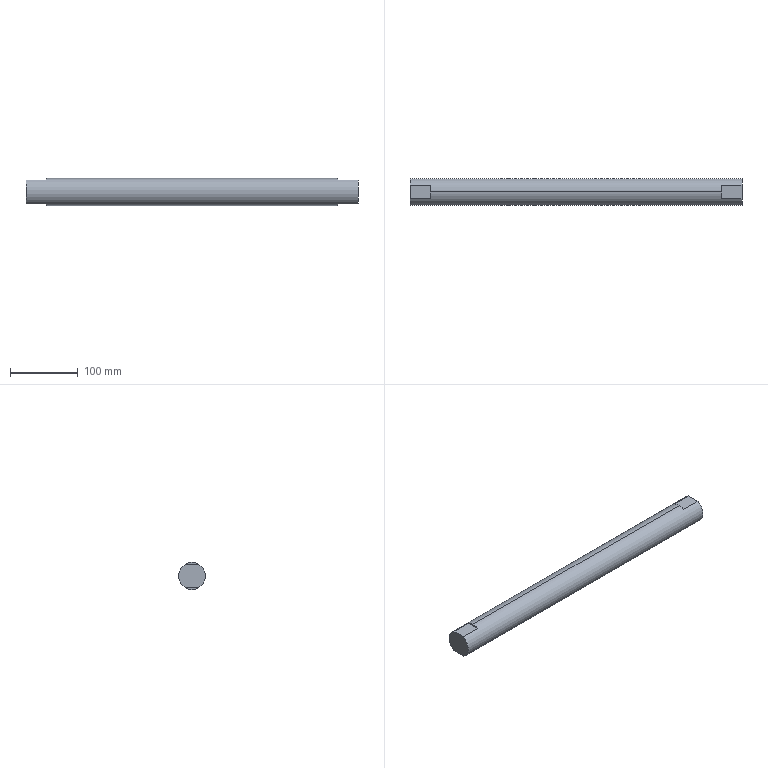Part | STEP file | Threading sliding shaft SGN-2-12 | 1 solid | 12 faces | box 490 x 40 x 40 mm | volume 611828 mm3 | plane 10 | cylinder 2 | commonest cylinder face diameters 40 x2
STEP:
#1=CARTESIAN_POINT('',(0.,0.,0.));
#2=DIRECTION('',(0.,0.,1.));
#3=DIRECTION('',(1.,0.,0.));
#4=AXIS2_PLACEMENT_3D('',#1,#2,#3);
#5=CARTESIAN_POINT('',(295.,9.682,-2.5));
#6=VERTEX_POINT('',#5);
#7=CARTESIAN_POINT('',(295.,0.,-5.));
#8=VERTEX_POINT('',#7);
#9=CARTESIAN_POINT('',(295.,0.,15.));
#10=DIRECTION('',(-1.,0.,0.));
#11=DIRECTION('',(0.,0.,-1.));
#12=AXIS2_PLACEMENT_3D('',#9,#10,#11);
#13=CIRCLE('',#12,20.);
#14=CARTESIAN_POINT('',(189.,0.,15.));
#15=DIRECTION('',(-1.,0.,0.));
#16=DIRECTION('',(0.,0.,1.));
#17=AXIS2_PLACEMENT_3D('',#14,#15,#16);
#18=CYLINDRICAL_SURFACE('',#17,20.);
#19=CARTESIAN_POINT('',(-3.142,-106.));
#20=DIRECTION('',(1.,0.));
#21=VECTOR('',#20,1.);
#22=LINE('',#19,#21);
#23=(GEOMETRIC_REPRESENTATION_CONTEXT(2)PARAMETRIC_REPRESENTATION_CONTEXT()REPRESENTATION_CONTEXT('',''));
#24=DEFINITIONAL_REPRESENTATION('',(#22),#23);
#25=PCURVE('',#18,#24);
#26=CARTESIAN_POINT('',(295.,0.,15.));
#27=DIRECTION('',(1.,0.,0.));
#28=DIRECTION('',(0.,0.,-1.));
#29=AXIS2_PLACEMENT_3D('',#26,#27,#28);
#30=PLANE('',#29);
#31=CARTESIAN_POINT('',(20.,0.));
#32=CARTESIAN_POINT('',(20.,-34.641));
#33=CARTESIAN_POINT('',(-10.,-17.321));
#34=CARTESIAN_POINT('',(-40.,0.));
#35=CARTESIAN_POINT('',(-10.,17.321));
#36=CARTESIAN_POINT('',(20.,34.641));
#37=CARTESIAN_POINT('',(20.,0.));
#38=(BOUNDED_CURVE()B_SPLINE_CURVE(2,(#31,#32,#33,#34,#35,#36,#37),.UNSPECIFIED.,.T.,.F.)B_SPLINE_CURVE_WITH_KNOTS((1,2,2,2,2,1),(-2.094,0.,2.094,4.189,6.283,8.378),.UNSPECIFIED.)CURVE()GEOMETRIC_REPRESENTATION_ITEM()RATIONAL_B_SPLINE_CURVE((1.,0.5,1.,0.5,1.,0.5,1.))REPRESENTATION_ITEM(''));
#39=(GEOMETRIC_REPRESENTATION_CONTEXT(2)PARAMETRIC_REPRESENTATION_CONTEXT()REPRESENTATION_CONTEXT('',''));
#40=DEFINITIONAL_REPRESENTATION('',(#38),#39);
#41=PCURVE('',#30,#40);
#42=SURFACE_CURVE('',#13,(#25,#41),.PCURVE_S1.);
#43=EDGE_CURVE('',#6,#8,#42,.T.);
#44=ORIENTED_EDGE('',*,*,#43,.T.);
#45=CARTESIAN_POINT('',(-135.,0.,-5.));
#46=VERTEX_POINT('',#45);
#47=CARTESIAN_POINT('',(189.,0.,-5.));
#48=DIRECTION('',(-1.,0.,0.));
#49=VECTOR('',#48,1.);
#50=LINE('',#47,#49);
#51=CARTESIAN_POINT('',(3.142,0.));
#52=DIRECTION('',(0.,1.));
#53=VECTOR('',#52,1.);
#54=LINE('',#51,#53);
#55=(GEOMETRIC_REPRESENTATION_CONTEXT(2)PARAMETRIC_REPRESENTATION_CONTEXT()REPRESENTATION_CONTEXT('',''));
#56=DEFINITIONAL_REPRESENTATION('',(#54),#55);
#57=PCURVE('',#18,#56);
#58=CARTESIAN_POINT('',(189.,0.,15.));
#59=DIRECTION('',(-1.,0.,0.));
#60=DIRECTION('',(0.,0.,1.));
#61=AXIS2_PLACEMENT_3D('',#58,#59,#60);
#62=CYLINDRICAL_SURFACE('',#61,20.);
#63=CARTESIAN_POINT('',(3.142,0.));
#64=DIRECTION('',(0.,1.));
#65=VECTOR('',#64,1.);
#66=LINE('',#63,#65);
#67=(GEOMETRIC_REPRESENTATION_CONTEXT(2)PARAMETRIC_REPRESENTATION_CONTEXT()REPRESENTATION_CONTEXT('',''));
#68=DEFINITIONAL_REPRESENTATION('',(#66),#67);
#69=PCURVE('',#62,#68);
#70=SURFACE_CURVE('',#50,(#57,#69),.PCURVE_S1.);
#71=EDGE_CURVE('',#8,#46,#70,.T.);
#72=ORIENTED_EDGE('',*,*,#71,.T.);
#73=CARTESIAN_POINT('',(-135.,9.682,-2.5));
#74=VERTEX_POINT('',#73);
#75=CARTESIAN_POINT('',(-135.,0.,15.));
#76=DIRECTION('',(1.,0.,0.));
#77=DIRECTION('',(0.,0.,1.));
#78=AXIS2_PLACEMENT_3D('',#75,#76,#77);
#79=CIRCLE('',#78,20.);
#80=CARTESIAN_POINT('',(6.283,324.));
#81=DIRECTION('',(-1.,0.));
#82=VECTOR('',#81,1.);
#83=LINE('',#80,#82);
#84=(GEOMETRIC_REPRESENTATION_CONTEXT(2)PARAMETRIC_REPRESENTATION_CONTEXT()REPRESENTATION_CONTEXT('',''));
#85=DEFINITIONAL_REPRESENTATION('',(#83),#84);
#86=PCURVE('',#18,#85);
#87=CARTESIAN_POINT('',(-135.,0.,15.));
#88=DIRECTION('',(-1.,0.,0.));
#89=DIRECTION('',(0.,0.,1.));
#90=AXIS2_PLACEMENT_3D('',#87,#88,#89);
#91=PLANE('',#90);
#92=CARTESIAN_POINT('',(20.,0.));
#93=CARTESIAN_POINT('',(20.,-34.641));
#94=CARTESIAN_POINT('',(-10.,-17.321));
#95=CARTESIAN_POINT('',(-40.,0.));
#96=CARTESIAN_POINT('',(-10.,17.321));
#97=CARTESIAN_POINT('',(20.,34.641));
#98=CARTESIAN_POINT('',(20.,0.));
#99=(BOUNDED_CURVE()B_SPLINE_CURVE(2,(#92,#93,#94,#95,#96,#97,#98),.UNSPECIFIED.,.T.,.F.)B_SPLINE_CURVE_WITH_KNOTS((1,2,2,2,2,1),(-2.094,0.,2.094,4.189,6.283,8.378),.UNSPECIFIED.)CURVE()GEOMETRIC_REPRESENTATION_ITEM()RATIONAL_B_SPLINE_CURVE((1.,0.5,1.,0.5,1.,0.5,1.))REPRESENTATION_ITEM(''));
#100=(GEOMETRIC_REPRESENTATION_CONTEXT(2)PARAMETRIC_REPRESENTATION_CONTEXT()REPRESENTATION_CONTEXT('',''));
#101=DEFINITIONAL_REPRESENTATION('',(#99),#100);
#102=PCURVE('',#91,#101);
#103=SURFACE_CURVE('',#79,(#86,#102),.PCURVE_S1.);
#104=EDGE_CURVE('',#46,#74,#103,.T.);
#105=ORIENTED_EDGE('',*,*,#104,.T.);
#106=CARTESIAN_POINT('',(-165.,9.682,-2.5));
#107=VERTEX_POINT('',#106);
#108=CARTESIAN_POINT('',(189.,9.682,-2.5));
#109=DIRECTION('',(-1.,0.,0.));
#110=VECTOR('',#109,1.);
#111=LINE('',#108,#110);
#112=CARTESIAN_POINT('',(2.636,0.));
#113=DIRECTION('',(0.,1.));
#114=VECTOR('',#113,1.);
#115=LINE('',#112,#114);
#116=(GEOMETRIC_REPRESENTATION_CONTEXT(2)PARAMETRIC_REPRESENTATION_CONTEXT()REPRESENTATION_CONTEXT('',''));
#117=DEFINITIONAL_REPRESENTATION('',(#115),#116);
#118=PCURVE('',#18,#117);
#119=CARTESIAN_POINT('',(-135.,-24.484,-2.5));
#120=DIRECTION('',(0.,0.,-1.));
#121=DIRECTION('',(-1.,0.,0.));
#122=AXIS2_PLACEMENT_3D('',#119,#120,#121);
#123=PLANE('',#122);
#124=CARTESIAN_POINT('',(-324.,34.167));
#125=DIRECTION('',(1.,0.));
#126=VECTOR('',#125,1.);
#127=LINE('',#124,#126);
#128=(GEOMETRIC_REPRESENTATION_CONTEXT(2)PARAMETRIC_REPRESENTATION_CONTEXT()REPRESENTATION_CONTEXT('',''));
#129=DEFINITIONAL_REPRESENTATION('',(#127),#128);
#130=PCURVE('',#123,#129);
#131=SURFACE_CURVE('',#111,(#118,#130),.PCURVE_S1.);
#132=EDGE_CURVE('',#74,#107,#131,.T.);
#133=ORIENTED_EDGE('',*,*,#132,.T.);
#134=CARTESIAN_POINT('',(-165.,9.682,32.5));
#135=VERTEX_POINT('',#134);
#136=CARTESIAN_POINT('',(-165.,0.,15.));
#137=DIRECTION('',(-1.,0.,0.));
#138=DIRECTION('',(0.,0.,1.));
#139=AXIS2_PLACEMENT_3D('',#136,#137,#138);
#140=CIRCLE('',#139,20.);
#141=CARTESIAN_POINT('',(0.,354.));
#142=DIRECTION('',(1.,0.));
#143=VECTOR('',#142,1.);
#144=LINE('',#141,#143);
#145=(GEOMETRIC_REPRESENTATION_CONTEXT(2)PARAMETRIC_REPRESENTATION_CONTEXT()REPRESENTATION_CONTEXT('',''));
#146=DEFINITIONAL_REPRESENTATION('',(#144),#145);
#147=PCURVE('',#18,#146);
#148=CARTESIAN_POINT('',(-165.,0.,15.));
#149=DIRECTION('',(-1.,0.,0.));
#150=DIRECTION('',(0.,0.,1.));
#151=AXIS2_PLACEMENT_3D('',#148,#149,#150);
#152=PLANE('',#151);
#153=CARTESIAN_POINT('',(0.,0.));
#154=DIRECTION('',(1.,0.));
#155=AXIS2_PLACEMENT_2D('',#153,#154);
#156=CIRCLE('',#155,20.);
#157=(GEOMETRIC_REPRESENTATION_CONTEXT(2)PARAMETRIC_REPRESENTATION_CONTEXT()REPRESENTATION_CONTEXT('',''));
#158=DEFINITIONAL_REPRESENTATION('',(#156),#157);
#159=PCURVE('',#152,#158);
#160=SURFACE_CURVE('',#140,(#147,#159),.PCURVE_S1.);
#161=EDGE_CURVE('',#135,#107,#160,.T.);
#162=ORIENTED_EDGE('',*,*,#161,.F.);
#163=CARTESIAN_POINT('',(-135.,9.682,32.5));
#164=VERTEX_POINT('',#163);
#165=CARTESIAN_POINT('',(189.,9.682,32.5));
#166=DIRECTION('',(1.,0.,0.));
#167=VECTOR('',#166,1.);
#168=LINE('',#165,#167);
#169=CARTESIAN_POINT('',(0.5054,0.));
#170=DIRECTION('',(0.,-1.));
#171=VECTOR('',#170,1.);
#172=LINE('',#169,#171);
#173=(GEOMETRIC_REPRESENTATION_CONTEXT(2)PARAMETRIC_REPRESENTATION_CONTEXT()REPRESENTATION_CONTEXT('',''));
#174=DEFINITIONAL_REPRESENTATION('',(#172),#173);
#175=PCURVE('',#18,#174);
#176=CARTESIAN_POINT('',(-135.,-24.484,32.5));
#177=DIRECTION('',(0.,0.,1.));
#178=DIRECTION('',(1.,0.,0.));
#179=AXIS2_PLACEMENT_3D('',#176,#177,#178);
#180=PLANE('',#179);
#181=CARTESIAN_POINT('',(324.,34.167));
#182=DIRECTION('',(1.,0.));
#183=VECTOR('',#182,1.);
#184=LINE('',#181,#183);
#185=(GEOMETRIC_REPRESENTATION_CONTEXT(2)PARAMETRIC_REPRESENTATION_CONTEXT()REPRESENTATION_CONTEXT('',''));
#186=DEFINITIONAL_REPRESENTATION('',(#184),#185);
#187=PCURVE('',#180,#186);
#188=SURFACE_CURVE('',#168,(#175,#187),.PCURVE_S1.);
#189=EDGE_CURVE('',#135,#164,#188,.T.);
#190=ORIENTED_EDGE('',*,*,#189,.T.);
#191=CARTESIAN_POINT('',(-135.,0.,35.));
#192=VERTEX_POINT('',#191);
#193=CARTESIAN_POINT('',(-135.,0.,15.));
#194=DIRECTION('',(1.,0.,0.));
#195=DIRECTION('',(0.,0.,1.));
#196=AXIS2_PLACEMENT_3D('',#193,#194,#195);
#197=CIRCLE('',#196,20.);
#198=CARTESIAN_POINT('',(6.283,324.));
#199=DIRECTION('',(-1.,0.));
#200=VECTOR('',#199,1.);
#201=LINE('',#198,#200);
#202=(GEOMETRIC_REPRESENTATION_CONTEXT(2)PARAMETRIC_REPRESENTATION_CONTEXT()REPRESENTATION_CONTEXT('',''));
#203=DEFINITIONAL_REPRESENTATION('',(#201),#202);
#204=PCURVE('',#18,#203);
#205=CARTESIAN_POINT('',(-135.,0.,15.));
#206=DIRECTION('',(-1.,0.,0.));
#207=DIRECTION('',(0.,0.,1.));
#208=AXIS2_PLACEMENT_3D('',#205,#206,#207);
#209=PLANE('',#208);
#210=CARTESIAN_POINT('',(20.,0.));
#211=CARTESIAN_POINT('',(20.,-34.641));
#212=CARTESIAN_POINT('',(-10.,-17.321));
#213=CARTESIAN_POINT('',(-40.,0.));
#214=CARTESIAN_POINT('',(-10.,17.321));
#215=CARTESIAN_POINT('',(20.,34.641));
#216=CARTESIAN_POINT('',(20.,0.));
#217=(BOUNDED_CURVE()B_SPLINE_CURVE(2,(#210,#211,#212,#213,#214,#215,#216),.UNSPECIFIED.,.T.,.F.)B_SPLINE_CURVE_WITH_KNOTS((1,2,2,2,2,1),(-2.094,0.,2.094,4.189,6.283,8.378),.UNSPECIFIED.)CURVE()GEOMETRIC_REPRESENTATION_ITEM()RATIONAL_B_SPLINE_CURVE((1.,0.5,1.,0.5,1.,0.5,1.))REPRESENTATION_ITEM(''));
#218=(GEOMETRIC_REPRESENTATION_CONTEXT(2)PARAMETRIC_REPRESENTATION_CONTEXT()REPRESENTATION_CONTEXT('',''));
#219=DEFINITIONAL_REPRESENTATION('',(#217),#218);
#220=PCURVE('',#209,#219);
#221=SURFACE_CURVE('',#197,(#204,#220),.PCURVE_S1.);
#222=EDGE_CURVE('',#164,#192,#221,.T.);
#223=ORIENTED_EDGE('',*,*,#222,.T.);
#224=CARTESIAN_POINT('',(295.,0.,35.));
#225=VERTEX_POINT('',#224);
#226=CARTESIAN_POINT('',(189.,0.,35.));
#227=DIRECTION('',(-1.,0.,0.));
#228=VECTOR('',#227,1.);
#229=LINE('',#226,#228);
#230=CARTESIAN_POINT('',(0.,0.));
#231=DIRECTION('',(0.,1.));
#232=VECTOR('',#231,1.);
#233=LINE('',#230,#232);
#234=(GEOMETRIC_REPRESENTATION_CONTEXT(2)PARAMETRIC_REPRESENTATION_CONTEXT()REPRESENTATION_CONTEXT('',''));
#235=DEFINITIONAL_REPRESENTATION('',(#233),#234);
#236=PCURVE('',#18,#235);
#237=CARTESIAN_POINT('',(6.283,0.));
#238=DIRECTION('',(0.,1.));
#239=VECTOR('',#238,1.);
#240=LINE('',#237,#239);
#241=(GEOMETRIC_REPRESENTATION_CONTEXT(2)PARAMETRIC_REPRESENTATION_CONTEXT()REPRESENTATION_CONTEXT('',''));
#242=DEFINITIONAL_REPRESENTATION('',(#240),#241);
#243=PCURVE('',#62,#242);
#244=SURFACE_CURVE('',#229,(#236,#243),.PCURVE_S1.);
#245=EDGE_CURVE('',#225,#192,#244,.T.);
#246=ORIENTED_EDGE('',*,*,#245,.F.);
#247=CARTESIAN_POINT('',(295.,9.682,32.5));
#248=VERTEX_POINT('',#247);
#249=CARTESIAN_POINT('',(295.,0.,15.));
#250=DIRECTION('',(-1.,0.,0.));
#251=DIRECTION('',(0.,0.,-1.));
#252=AXIS2_PLACEMENT_3D('',#249,#250,#251);
#253=CIRCLE('',#252,20.);
#254=CARTESIAN_POINT('',(-3.142,-106.));
#255=DIRECTION('',(1.,0.));
#256=VECTOR('',#255,1.);
#257=LINE('',#254,#256);
#258=(GEOMETRIC_REPRESENTATION_CONTEXT(2)PARAMETRIC_REPRESENTATION_CONTEXT()REPRESENTATION_CONTEXT('',''));
#259=DEFINITIONAL_REPRESENTATION('',(#257),#258);
#260=PCURVE('',#18,#259);
#261=CARTESIAN_POINT('',(295.,0.,15.));
#262=DIRECTION('',(1.,0.,0.));
#263=DIRECTION('',(0.,0.,-1.));
#264=AXIS2_PLACEMENT_3D('',#261,#262,#263);
#265=PLANE('',#264);
#266=CARTESIAN_POINT('',(20.,0.));
#267=CARTESIAN_POINT('',(20.,-34.641));
#268=CARTESIAN_POINT('',(-10.,-17.321));
#269=CARTESIAN_POINT('',(-40.,0.));
#270=CARTESIAN_POINT('',(-10.,17.321));
#271=CARTESIAN_POINT('',(20.,34.641));
#272=CARTESIAN_POINT('',(20.,0.));
#273=(BOUNDED_CURVE()B_SPLINE_CURVE(2,(#266,#267,#268,#269,#270,#271,#272),.UNSPECIFIED.,.T.,.F.)B_SPLINE_CURVE_WITH_KNOTS((1,2,2,2,2,1),(-2.094,0.,2.094,4.189,6.283,8.378),.UNSPECIFIED.)CURVE()GEOMETRIC_REPRESENTATION_ITEM()RATIONAL_B_SPLINE_CURVE((1.,0.5,1.,0.5,1.,0.5,1.))REPRESENTATION_ITEM(''));
#274=(GEOMETRIC_REPRESENTATION_CONTEXT(2)PARAMETRIC_REPRESENTATION_CONTEXT()REPRESENTATION_CONTEXT('',''));
#275=DEFINITIONAL_REPRESENTATION('',(#273),#274);
#276=PCURVE('',#265,#275);
#277=SURFACE_CURVE('',#253,(#260,#276),.PCURVE_S1.);
#278=EDGE_CURVE('',#225,#248,#277,.T.);
#279=ORIENTED_EDGE('',*,*,#278,.T.);
#280=CARTESIAN_POINT('',(325.,9.682,32.5));
#281=VERTEX_POINT('',#280);
#282=CARTESIAN_POINT('',(189.,9.682,32.5));
#283=DIRECTION('',(1.,0.,0.));
#284=VECTOR('',#283,1.);
#285=LINE('',#282,#284);
#286=CARTESIAN_POINT('',(0.5054,0.));
#287=DIRECTION('',(0.,-1.));
#288=VECTOR('',#287,1.);
#289=LINE('',#286,#288);
#290=(GEOMETRIC_REPRESENTATION_CONTEXT(2)PARAMETRIC_REPRESENTATION_CONTEXT()REPRESENTATION_CONTEXT('',''));
#291=DEFINITIONAL_REPRESENTATION('',(#289),#290);
#292=PCURVE('',#18,#291);
#293=CARTESIAN_POINT('',(295.,-22.774,32.5));
#294=DIRECTION('',(0.,0.,1.));
#295=DIRECTION('',(1.,0.,0.));
#296=AXIS2_PLACEMENT_3D('',#293,#294,#295);
#297=PLANE('',#296);
#298=CARTESIAN_POINT('',(-106.,32.457));
#299=DIRECTION('',(1.,0.));
#300=VECTOR('',#299,1.);
#301=LINE('',#298,#300);
#302=(GEOMETRIC_REPRESENTATION_CONTEXT(2)PARAMETRIC_REPRESENTATION_CONTEXT()REPRESENTATION_CONTEXT('',''));
#303=DEFINITIONAL_REPRESENTATION('',(#301),#302);
#304=PCURVE('',#297,#303);
#305=SURFACE_CURVE('',#285,(#292,#304),.PCURVE_S1.);
#306=EDGE_CURVE('',#248,#281,#305,.T.);
#307=ORIENTED_EDGE('',*,*,#306,.T.);
#308=CARTESIAN_POINT('',(325.,9.682,-2.5));
#309=VERTEX_POINT('',#308);
#310=CARTESIAN_POINT('',(325.,0.,15.));
#311=DIRECTION('',(1.,0.,0.));
#312=DIRECTION('',(0.,0.,-1.));
#313=AXIS2_PLACEMENT_3D('',#310,#311,#312);
#314=CIRCLE('',#313,20.);
#315=CARTESIAN_POINT('',(3.142,-136.));
#316=DIRECTION('',(-1.,0.));
#317=VECTOR('',#316,1.);
#318=LINE('',#315,#317);
#319=(GEOMETRIC_REPRESENTATION_CONTEXT(2)PARAMETRIC_REPRESENTATION_CONTEXT()REPRESENTATION_CONTEXT('',''));
#320=DEFINITIONAL_REPRESENTATION('',(#318),#319);
#321=PCURVE('',#18,#320);
#322=CARTESIAN_POINT('',(325.,0.,15.));
#323=DIRECTION('',(1.,0.,0.));
#324=DIRECTION('',(0.,0.,-1.));
#325=AXIS2_PLACEMENT_3D('',#322,#323,#324);
#326=PLANE('',#325);
#327=CARTESIAN_POINT('',(0.,0.));
#328=DIRECTION('',(1.,0.));
#329=AXIS2_PLACEMENT_2D('',#327,#328);
#330=CIRCLE('',#329,20.);
#331=(GEOMETRIC_REPRESENTATION_CONTEXT(2)PARAMETRIC_REPRESENTATION_CONTEXT()REPRESENTATION_CONTEXT('',''));
#332=DEFINITIONAL_REPRESENTATION('',(#330),#331);
#333=PCURVE('',#326,#332);
#334=SURFACE_CURVE('',#314,(#321,#333),.PCURVE_S1.);
#335=EDGE_CURVE('',#309,#281,#334,.T.);
#336=ORIENTED_EDGE('',*,*,#335,.F.);
#337=CARTESIAN_POINT('',(189.,9.682,-2.5));
#338=DIRECTION('',(-1.,0.,0.));
#339=VECTOR('',#338,1.);
#340=LINE('',#337,#339);
#341=CARTESIAN_POINT('',(2.636,0.));
#342=DIRECTION('',(0.,1.));
#343=VECTOR('',#342,1.);
#344=LINE('',#341,#343);
#345=(GEOMETRIC_REPRESENTATION_CONTEXT(2)PARAMETRIC_REPRESENTATION_CONTEXT()REPRESENTATION_CONTEXT('',''));
#346=DEFINITIONAL_REPRESENTATION('',(#344),#345);
#347=PCURVE('',#18,#346);
#348=CARTESIAN_POINT('',(295.,-22.774,-2.5));
#349=DIRECTION('',(0.,0.,-1.));
#350=DIRECTION('',(-1.,0.,0.));
#351=AXIS2_PLACEMENT_3D('',#348,#349,#350);
#352=PLANE('',#351);
#353=CARTESIAN_POINT('',(106.,32.457));
#354=DIRECTION('',(1.,0.));
#355=VECTOR('',#354,1.);
#356=LINE('',#353,#355);
#357=(GEOMETRIC_REPRESENTATION_CONTEXT(2)PARAMETRIC_REPRESENTATION_CONTEXT()REPRESENTATION_CONTEXT('',''));
#358=DEFINITIONAL_REPRESENTATION('',(#356),#357);
#359=PCURVE('',#352,#358);
#360=SURFACE_CURVE('',#340,(#347,#359),.PCURVE_S1.);
#361=EDGE_CURVE('',#309,#6,#360,.T.);
#362=ORIENTED_EDGE('',*,*,#361,.T.);
#363=EDGE_LOOP('',(#44,#72,#105,#133,#162,#190,#223,#246,#279,#307,#336,#362));
#364=FACE_BOUND('',#363,.T.);
#365=ADVANCED_FACE('',(#364),#18,.T.);
#366=ORIENTED_EDGE('',*,*,#71,.F.);
#367=CARTESIAN_POINT('',(295.,-9.682,-2.5));
#368=VERTEX_POINT('',#367);
#369=CARTESIAN_POINT('',(295.,0.,15.));
#370=DIRECTION('',(-1.,0.,0.));
#371=DIRECTION('',(0.,0.,-1.));
#372=AXIS2_PLACEMENT_3D('',#369,#370,#371);
#373=CIRCLE('',#372,20.);
#374=CARTESIAN_POINT('',(3.142,-106.));
#375=DIRECTION('',(1.,0.));
#376=VECTOR('',#375,1.);
#377=LINE('',#374,#376);
#378=(GEOMETRIC_REPRESENTATION_CONTEXT(2)PARAMETRIC_REPRESENTATION_CONTEXT()REPRESENTATION_CONTEXT('',''));
#379=DEFINITIONAL_REPRESENTATION('',(#377),#378);
#380=PCURVE('',#62,#379);
#381=CARTESIAN_POINT('',(20.,0.));
#382=CARTESIAN_POINT('',(20.,-34.641));
#383=CARTESIAN_POINT('',(-10.,-17.321));
#384=CARTESIAN_POINT('',(-40.,0.));
#385=CARTESIAN_POINT('',(-10.,17.321));
#386=CARTESIAN_POINT('',(20.,34.641));
#387=CARTESIAN_POINT('',(20.,0.));
#388=(BOUNDED_CURVE()B_SPLINE_CURVE(2,(#381,#382,#383,#384,#385,#386,#387),.UNSPECIFIED.,.T.,.F.)B_SPLINE_CURVE_WITH_KNOTS((1,2,2,2,2,1),(-2.094,0.,2.094,4.189,6.283,8.378),.UNSPECIFIED.)CURVE()GEOMETRIC_REPRESENTATION_ITEM()RATIONAL_B_SPLINE_CURVE((1.,0.5,1.,0.5,1.,0.5,1.))REPRESENTATION_ITEM(''));
#389=(GEOMETRIC_REPRESENTATION_CONTEXT(2)PARAMETRIC_REPRESENTATION_CONTEXT()REPRESENTATION_CONTEXT('',''));
#390=DEFINITIONAL_REPRESENTATION('',(#388),#389);
#391=PCURVE('',#30,#390);
#392=SURFACE_CURVE('',#373,(#380,#391),.PCURVE_S1.);
#393=EDGE_CURVE('',#8,#368,#392,.T.);
#394=ORIENTED_EDGE('',*,*,#393,.T.);
#395=CARTESIAN_POINT('',(325.,-9.682,-2.5));
#396=VERTEX_POINT('',#395);
#397=CARTESIAN_POINT('',(189.,-9.682,-2.5));
#398=DIRECTION('',(1.,0.,0.));
#399=VECTOR('',#398,1.);
#400=LINE('',#397,#399);
#401=CARTESIAN_POINT('',(3.647,0.));
#402=DIRECTION('',(0.,-1.));
#403=VECTOR('',#402,1.);
#404=LINE('',#401,#403);
#405=(GEOMETRIC_REPRESENTATION_CONTEXT(2)PARAMETRIC_REPRESENTATION_CONTEXT()REPRESENTATION_CONTEXT('',''));
#406=DEFINITIONAL_REPRESENTATION('',(#404),#405);
#407=PCURVE('',#62,#406);
#408=CARTESIAN_POINT('',(106.,13.092));
#409=DIRECTION('',(-1.,0.));
#410=VECTOR('',#409,1.);
#411=LINE('',#408,#410);
#412=(GEOMETRIC_REPRESENTATION_CONTEXT(2)PARAMETRIC_REPRESENTATION_CONTEXT()REPRESENTATION_CONTEXT('',''));
#413=DEFINITIONAL_REPRESENTATION('',(#411),#412);
#414=PCURVE('',#352,#413);
#415=SURFACE_CURVE('',#400,(#407,#414),.PCURVE_S1.);
#416=EDGE_CURVE('',#368,#396,#415,.T.);
#417=ORIENTED_EDGE('',*,*,#416,.T.);
#418=CARTESIAN_POINT('',(325.,-9.682,32.5));
#419=VERTEX_POINT('',#418);
#420=CARTESIAN_POINT('',(325.,0.,15.));
#421=DIRECTION('',(1.,0.,0.));
#422=DIRECTION('',(0.,0.,-1.));
#423=AXIS2_PLACEMENT_3D('',#420,#421,#422);
#424=CIRCLE('',#423,20.);
#425=CARTESIAN_POINT('',(9.425,-136.));
#426=DIRECTION('',(-1.,0.));
#427=VECTOR('',#426,1.);
#428=LINE('',#425,#427);
#429=(GEOMETRIC_REPRESENTATION_CONTEXT(2)PARAMETRIC_REPRESENTATION_CONTEXT()REPRESENTATION_CONTEXT('',''));
#430=DEFINITIONAL_REPRESENTATION('',(#428),#429);
#431=PCURVE('',#62,#430);
#432=CARTESIAN_POINT('',(0.,0.));
#433=DIRECTION('',(1.,0.));
#434=AXIS2_PLACEMENT_2D('',#432,#433);
#435=CIRCLE('',#434,20.);
#436=(GEOMETRIC_REPRESENTATION_CONTEXT(2)PARAMETRIC_REPRESENTATION_CONTEXT()REPRESENTATION_CONTEXT('',''));
#437=DEFINITIONAL_REPRESENTATION('',(#435),#436);
#438=PCURVE('',#326,#437);
#439=SURFACE_CURVE('',#424,(#431,#438),.PCURVE_S1.);
#440=EDGE_CURVE('',#419,#396,#439,.T.);
#441=ORIENTED_EDGE('',*,*,#440,.F.);
#442=CARTESIAN_POINT('',(295.,-9.682,32.5));
#443=VERTEX_POINT('',#442);
#444=CARTESIAN_POINT('',(189.,-9.682,32.5));
#445=DIRECTION('',(-1.,0.,0.));
#446=VECTOR('',#445,1.);
#447=LINE('',#444,#446);
#448=CARTESIAN_POINT('',(5.778,0.));
#449=DIRECTION('',(0.,1.));
#450=VECTOR('',#449,1.);
#451=LINE('',#448,#450);
#452=(GEOMETRIC_REPRESENTATION_CONTEXT(2)PARAMETRIC_REPRESENTATION_CONTEXT()REPRESENTATION_CONTEXT('',''));
#453=DEFINITIONAL_REPRESENTATION('',(#451),#452);
#454=PCURVE('',#62,#453);
#455=CARTESIAN_POINT('',(-106.,13.092));
#456=DIRECTION('',(-1.,0.));
#457=VECTOR('',#456,1.);
#458=LINE('',#455,#457);
#459=(GEOMETRIC_REPRESENTATION_CONTEXT(2)PARAMETRIC_REPRESENTATION_CONTEXT()REPRESENTATION_CONTEXT('',''));
#460=DEFINITIONAL_REPRESENTATION('',(#458),#459);
#461=PCURVE('',#297,#460);
#462=SURFACE_CURVE('',#447,(#454,#461),.PCURVE_S1.);
#463=EDGE_CURVE('',#419,#443,#462,.T.);
#464=ORIENTED_EDGE('',*,*,#463,.T.);
#465=CARTESIAN_POINT('',(295.,0.,15.));
#466=DIRECTION('',(-1.,0.,0.));
#467=DIRECTION('',(0.,0.,-1.));
#468=AXIS2_PLACEMENT_3D('',#465,#466,#467);
#469=CIRCLE('',#468,20.);
#470=CARTESIAN_POINT('',(3.142,-106.));
#471=DIRECTION('',(1.,0.));
#472=VECTOR('',#471,1.);
#473=LINE('',#470,#472);
#474=(GEOMETRIC_REPRESENTATION_CONTEXT(2)PARAMETRIC_REPRESENTATION_CONTEXT()REPRESENTATION_CONTEXT('',''));
#475=DEFINITIONAL_REPRESENTATION('',(#473),#474);
#476=PCURVE('',#62,#475);
#477=CARTESIAN_POINT('',(20.,0.));
#478=CARTESIAN_POINT('',(20.,-34.641));
#479=CARTESIAN_POINT('',(-10.,-17.321));
#480=CARTESIAN_POINT('',(-40.,0.));
#481=CARTESIAN_POINT('',(-10.,17.321));
#482=CARTESIAN_POINT('',(20.,34.641));
#483=CARTESIAN_POINT('',(20.,0.));
#484=(BOUNDED_CURVE()B_SPLINE_CURVE(2,(#477,#478,#479,#480,#481,#482,#483),.UNSPECIFIED.,.T.,.F.)B_SPLINE_CURVE_WITH_KNOTS((1,2,2,2,2,1),(-2.094,0.,2.094,4.189,6.283,8.378),.UNSPECIFIED.)CURVE()GEOMETRIC_REPRESENTATION_ITEM()RATIONAL_B_SPLINE_CURVE((1.,0.5,1.,0.5,1.,0.5,1.))REPRESENTATION_ITEM(''));
#485=(GEOMETRIC_REPRESENTATION_CONTEXT(2)PARAMETRIC_REPRESENTATION_CONTEXT()REPRESENTATION_CONTEXT('',''));
#486=DEFINITIONAL_REPRESENTATION('',(#484),#485);
#487=PCURVE('',#265,#486);
#488=SURFACE_CURVE('',#469,(#476,#487),.PCURVE_S1.);
#489=EDGE_CURVE('',#443,#225,#488,.T.);
#490=ORIENTED_EDGE('',*,*,#489,.T.);
#491=ORIENTED_EDGE('',*,*,#245,.T.);
#492=CARTESIAN_POINT('',(-135.,-9.682,32.5));
#493=VERTEX_POINT('',#492);
#494=CARTESIAN_POINT('',(-135.,0.,15.));
#495=DIRECTION('',(1.,0.,0.));
#496=DIRECTION('',(0.,0.,1.));
#497=AXIS2_PLACEMENT_3D('',#494,#495,#496);
#498=CIRCLE('',#497,20.);
#499=CARTESIAN_POINT('',(6.283,324.));
#500=DIRECTION('',(-1.,0.));
#501=VECTOR('',#500,1.);
#502=LINE('',#499,#501);
#503=(GEOMETRIC_REPRESENTATION_CONTEXT(2)PARAMETRIC_REPRESENTATION_CONTEXT()REPRESENTATION_CONTEXT('',''));
#504=DEFINITIONAL_REPRESENTATION('',(#502),#503);
#505=PCURVE('',#62,#504);
#506=CARTESIAN_POINT('',(20.,0.));
#507=CARTESIAN_POINT('',(20.,-34.641));
#508=CARTESIAN_POINT('',(-10.,-17.321));
#509=CARTESIAN_POINT('',(-40.,0.));
#510=CARTESIAN_POINT('',(-10.,17.321));
#511=CARTESIAN_POINT('',(20.,34.641));
#512=CARTESIAN_POINT('',(20.,0.));
#513=(BOUNDED_CURVE()B_SPLINE_CURVE(2,(#506,#507,#508,#509,#510,#511,#512),.UNSPECIFIED.,.T.,.F.)B_SPLINE_CURVE_WITH_KNOTS((1,2,2,2,2,1),(-2.094,0.,2.094,4.189,6.283,8.378),.UNSPECIFIED.)CURVE()GEOMETRIC_REPRESENTATION_ITEM()RATIONAL_B_SPLINE_CURVE((1.,0.5,1.,0.5,1.,0.5,1.))REPRESENTATION_ITEM(''));
#514=(GEOMETRIC_REPRESENTATION_CONTEXT(2)PARAMETRIC_REPRESENTATION_CONTEXT()REPRESENTATION_CONTEXT('',''));
#515=DEFINITIONAL_REPRESENTATION('',(#513),#514);
#516=PCURVE('',#209,#515);
#517=SURFACE_CURVE('',#498,(#505,#516),.PCURVE_S1.);
#518=EDGE_CURVE('',#192,#493,#517,.T.);
#519=ORIENTED_EDGE('',*,*,#518,.T.);
#520=CARTESIAN_POINT('',(-165.,-9.682,32.5));
#521=VERTEX_POINT('',#520);
#522=CARTESIAN_POINT('',(189.,-9.682,32.5));
#523=DIRECTION('',(-1.,0.,0.));
#524=VECTOR('',#523,1.);
#525=LINE('',#522,#524);
#526=CARTESIAN_POINT('',(5.778,0.));
#527=DIRECTION('',(0.,1.));
#528=VECTOR('',#527,1.);
#529=LINE('',#526,#528);
#530=(GEOMETRIC_REPRESENTATION_CONTEXT(2)PARAMETRIC_REPRESENTATION_CONTEXT()REPRESENTATION_CONTEXT('',''));
#531=DEFINITIONAL_REPRESENTATION('',(#529),#530);
#532=PCURVE('',#62,#531);
#533=CARTESIAN_POINT('',(324.,14.802));
#534=DIRECTION('',(-1.,0.));
#535=VECTOR('',#534,1.);
#536=LINE('',#533,#535);
#537=(GEOMETRIC_REPRESENTATION_CONTEXT(2)PARAMETRIC_REPRESENTATION_CONTEXT()REPRESENTATION_CONTEXT('',''));
#538=DEFINITIONAL_REPRESENTATION('',(#536),#537);
#539=PCURVE('',#180,#538);
#540=SURFACE_CURVE('',#525,(#532,#539),.PCURVE_S1.);
#541=EDGE_CURVE('',#493,#521,#540,.T.);
#542=ORIENTED_EDGE('',*,*,#541,.T.);
#543=CARTESIAN_POINT('',(-165.,-9.682,-2.5));
#544=VERTEX_POINT('',#543);
#545=CARTESIAN_POINT('',(-165.,0.,15.));
#546=DIRECTION('',(-1.,0.,0.));
#547=DIRECTION('',(0.,0.,1.));
#548=AXIS2_PLACEMENT_3D('',#545,#546,#547);
#549=CIRCLE('',#548,20.);
#550=CARTESIAN_POINT('',(0.,354.));
#551=DIRECTION('',(1.,0.));
#552=VECTOR('',#551,1.);
#553=LINE('',#550,#552);
#554=(GEOMETRIC_REPRESENTATION_CONTEXT(2)PARAMETRIC_REPRESENTATION_CONTEXT()REPRESENTATION_CONTEXT('',''));
#555=DEFINITIONAL_REPRESENTATION('',(#553),#554);
#556=PCURVE('',#62,#555);
#557=CARTESIAN_POINT('',(0.,0.));
#558=DIRECTION('',(1.,0.));
#559=AXIS2_PLACEMENT_2D('',#557,#558);
#560=CIRCLE('',#559,20.);
#561=(GEOMETRIC_REPRESENTATION_CONTEXT(2)PARAMETRIC_REPRESENTATION_CONTEXT()REPRESENTATION_CONTEXT('',''));
#562=DEFINITIONAL_REPRESENTATION('',(#560),#561);
#563=PCURVE('',#152,#562);
#564=SURFACE_CURVE('',#549,(#556,#563),.PCURVE_S1.);
#565=EDGE_CURVE('',#544,#521,#564,.T.);
#566=ORIENTED_EDGE('',*,*,#565,.F.);
#567=CARTESIAN_POINT('',(-135.,-9.682,-2.5));
#568=VERTEX_POINT('',#567);
#569=CARTESIAN_POINT('',(189.,-9.682,-2.5));
#570=DIRECTION('',(1.,0.,0.));
#571=VECTOR('',#570,1.);
#572=LINE('',#569,#571);
#573=CARTESIAN_POINT('',(3.647,0.));
#574=DIRECTION('',(0.,-1.));
#575=VECTOR('',#574,1.);
#576=LINE('',#573,#575);
#577=(GEOMETRIC_REPRESENTATION_CONTEXT(2)PARAMETRIC_REPRESENTATION_CONTEXT()REPRESENTATION_CONTEXT('',''));
#578=DEFINITIONAL_REPRESENTATION('',(#576),#577);
#579=PCURVE('',#62,#578);
#580=CARTESIAN_POINT('',(-324.,14.802));
#581=DIRECTION('',(-1.,0.));
#582=VECTOR('',#581,1.);
#583=LINE('',#580,#582);
#584=(GEOMETRIC_REPRESENTATION_CONTEXT(2)PARAMETRIC_REPRESENTATION_CONTEXT()REPRESENTATION_CONTEXT('',''));
#585=DEFINITIONAL_REPRESENTATION('',(#583),#584);
#586=PCURVE('',#123,#585);
#587=SURFACE_CURVE('',#572,(#579,#586),.PCURVE_S1.);
#588=EDGE_CURVE('',#544,#568,#587,.T.);
#589=ORIENTED_EDGE('',*,*,#588,.T.);
#590=CARTESIAN_POINT('',(-135.,0.,15.));
#591=DIRECTION('',(1.,0.,0.));
#592=DIRECTION('',(0.,0.,1.));
#593=AXIS2_PLACEMENT_3D('',#590,#591,#592);
#594=CIRCLE('',#593,20.);
#595=CARTESIAN_POINT('',(6.283,324.));
#596=DIRECTION('',(-1.,0.));
#597=VECTOR('',#596,1.);
#598=LINE('',#595,#597);
#599=(GEOMETRIC_REPRESENTATION_CONTEXT(2)PARAMETRIC_REPRESENTATION_CONTEXT()REPRESENTATION_CONTEXT('',''));
#600=DEFINITIONAL_REPRESENTATION('',(#598),#599);
#601=PCURVE('',#62,#600);
#602=CARTESIAN_POINT('',(20.,0.));
#603=CARTESIAN_POINT('',(20.,-34.641));
#604=CARTESIAN_POINT('',(-10.,-17.321));
#605=CARTESIAN_POINT('',(-40.,0.));
#606=CARTESIAN_POINT('',(-10.,17.321));
#607=CARTESIAN_POINT('',(20.,34.641));
#608=CARTESIAN_POINT('',(20.,0.));
#609=(BOUNDED_CURVE()B_SPLINE_CURVE(2,(#602,#603,#604,#605,#606,#607,#608),.UNSPECIFIED.,.T.,.F.)B_SPLINE_CURVE_WITH_KNOTS((1,2,2,2,2,1),(-2.094,0.,2.094,4.189,6.283,8.378),.UNSPECIFIED.)CURVE()GEOMETRIC_REPRESENTATION_ITEM()RATIONAL_B_SPLINE_CURVE((1.,0.5,1.,0.5,1.,0.5,1.))REPRESENTATION_ITEM(''));
#610=(GEOMETRIC_REPRESENTATION_CONTEXT(2)PARAMETRIC_REPRESENTATION_CONTEXT()REPRESENTATION_CONTEXT('',''));
#611=DEFINITIONAL_REPRESENTATION('',(#609),#610);
#612=PCURVE('',#91,#611);
#613=SURFACE_CURVE('',#594,(#601,#612),.PCURVE_S1.);
#614=EDGE_CURVE('',#568,#46,#613,.T.);
#615=ORIENTED_EDGE('',*,*,#614,.T.);
#616=EDGE_LOOP('',(#366,#394,#417,#441,#464,#490,#491,#519,#542,#566,#589,#615));
#617=FACE_BOUND('',#616,.T.);
#618=ADVANCED_FACE('',(#617),#62,.T.);
#619=ORIENTED_EDGE('',*,*,#565,.T.);
#620=CARTESIAN_POINT('',(-165.,0.,32.5));
#621=DIRECTION('',(0.,1.,0.));
#622=VECTOR('',#621,1.);
#623=LINE('',#620,#622);
#624=CARTESIAN_POINT('',(17.5,0.));
#625=DIRECTION('',(0.,1.));
#626=VECTOR('',#625,1.);
#627=LINE('',#624,#626);
#628=(GEOMETRIC_REPRESENTATION_CONTEXT(2)PARAMETRIC_REPRESENTATION_CONTEXT()REPRESENTATION_CONTEXT('',''));
#629=DEFINITIONAL_REPRESENTATION('',(#627),#628);
#630=PCURVE('',#152,#629);
#631=CARTESIAN_POINT('',(-30.,24.484));
#632=DIRECTION('',(0.,1.));
#633=VECTOR('',#632,1.);
#634=LINE('',#631,#633);
#635=(GEOMETRIC_REPRESENTATION_CONTEXT(2)PARAMETRIC_REPRESENTATION_CONTEXT()REPRESENTATION_CONTEXT('',''));
#636=DEFINITIONAL_REPRESENTATION('',(#634),#635);
#637=PCURVE('',#180,#636);
#638=SURFACE_CURVE('',#623,(#630,#637),.PCURVE_S1.);
#639=EDGE_CURVE('',#521,#135,#638,.T.);
#640=ORIENTED_EDGE('',*,*,#639,.T.);
#641=ORIENTED_EDGE('',*,*,#161,.T.);
#642=CARTESIAN_POINT('',(-165.,0.,-2.5));
#643=DIRECTION('',(0.,-1.,0.));
#644=VECTOR('',#643,1.);
#645=LINE('',#642,#644);
#646=CARTESIAN_POINT('',(-17.5,0.));
#647=DIRECTION('',(0.,-1.));
#648=VECTOR('',#647,1.);
#649=LINE('',#646,#648);
#650=(GEOMETRIC_REPRESENTATION_CONTEXT(2)PARAMETRIC_REPRESENTATION_CONTEXT()REPRESENTATION_CONTEXT('',''));
#651=DEFINITIONAL_REPRESENTATION('',(#649),#650);
#652=PCURVE('',#152,#651);
#653=CARTESIAN_POINT('',(30.,24.484));
#654=DIRECTION('',(0.,-1.));
#655=VECTOR('',#654,1.);
#656=LINE('',#653,#655);
#657=(GEOMETRIC_REPRESENTATION_CONTEXT(2)PARAMETRIC_REPRESENTATION_CONTEXT()REPRESENTATION_CONTEXT('',''));
#658=DEFINITIONAL_REPRESENTATION('',(#656),#657);
#659=PCURVE('',#123,#658);
#660=SURFACE_CURVE('',#645,(#652,#659),.PCURVE_S1.);
#661=EDGE_CURVE('',#107,#544,#660,.T.);
#662=ORIENTED_EDGE('',*,*,#661,.T.);
#663=EDGE_LOOP('',(#619,#640,#641,#662));
#664=FACE_BOUND('',#663,.T.);
#665=ADVANCED_FACE('',(#664),#152,.T.);
#666=ORIENTED_EDGE('',*,*,#440,.T.);
#667=CARTESIAN_POINT('',(325.,0.,-2.5));
#668=DIRECTION('',(0.,1.,0.));
#669=VECTOR('',#668,1.);
#670=LINE('',#667,#669);
#671=CARTESIAN_POINT('',(17.5,0.));
#672=DIRECTION('',(0.,1.));
#673=VECTOR('',#672,1.);
#674=LINE('',#671,#673);
#675=(GEOMETRIC_REPRESENTATION_CONTEXT(2)PARAMETRIC_REPRESENTATION_CONTEXT()REPRESENTATION_CONTEXT('',''));
#676=DEFINITIONAL_REPRESENTATION('',(#674),#675);
#677=PCURVE('',#326,#676);
#678=CARTESIAN_POINT('',(-30.,22.774));
#679=DIRECTION('',(0.,1.));
#680=VECTOR('',#679,1.);
#681=LINE('',#678,#680);
#682=(GEOMETRIC_REPRESENTATION_CONTEXT(2)PARAMETRIC_REPRESENTATION_CONTEXT()REPRESENTATION_CONTEXT('',''));
#683=DEFINITIONAL_REPRESENTATION('',(#681),#682);
#684=PCURVE('',#352,#683);
#685=SURFACE_CURVE('',#670,(#677,#684),.PCURVE_S1.);
#686=EDGE_CURVE('',#396,#309,#685,.T.);
#687=ORIENTED_EDGE('',*,*,#686,.T.);
#688=ORIENTED_EDGE('',*,*,#335,.T.);
#689=CARTESIAN_POINT('',(325.,0.,32.5));
#690=DIRECTION('',(0.,-1.,0.));
#691=VECTOR('',#690,1.);
#692=LINE('',#689,#691);
#693=CARTESIAN_POINT('',(-17.5,0.));
#694=DIRECTION('',(0.,-1.));
#695=VECTOR('',#694,1.);
#696=LINE('',#693,#695);
#697=(GEOMETRIC_REPRESENTATION_CONTEXT(2)PARAMETRIC_REPRESENTATION_CONTEXT()REPRESENTATION_CONTEXT('',''));
#698=DEFINITIONAL_REPRESENTATION('',(#696),#697);
#699=PCURVE('',#326,#698);
#700=CARTESIAN_POINT('',(30.,22.774));
#701=DIRECTION('',(0.,-1.));
#702=VECTOR('',#701,1.);
#703=LINE('',#700,#702);
#704=(GEOMETRIC_REPRESENTATION_CONTEXT(2)PARAMETRIC_REPRESENTATION_CONTEXT()REPRESENTATION_CONTEXT('',''));
#705=DEFINITIONAL_REPRESENTATION('',(#703),#704);
#706=PCURVE('',#297,#705);
#707=SURFACE_CURVE('',#692,(#699,#706),.PCURVE_S1.);
#708=EDGE_CURVE('',#281,#419,#707,.T.);
#709=ORIENTED_EDGE('',*,*,#708,.T.);
#710=EDGE_LOOP('',(#666,#687,#688,#709));
#711=FACE_BOUND('',#710,.T.);
#712=ADVANCED_FACE('',(#711),#326,.T.);
#713=CARTESIAN_POINT('',(295.,-22.774,32.5));
#714=DIRECTION('',(0.,-1.,0.));
#715=VECTOR('',#714,1.);
#716=LINE('',#713,#715);
#717=CARTESIAN_POINT('',(0.,0.));
#718=DIRECTION('',(0.,-1.));
#719=VECTOR('',#718,1.);
#720=LINE('',#717,#719);
#721=(GEOMETRIC_REPRESENTATION_CONTEXT(2)PARAMETRIC_REPRESENTATION_CONTEXT()REPRESENTATION_CONTEXT('',''));
#722=DEFINITIONAL_REPRESENTATION('',(#720),#721);
#723=PCURVE('',#297,#722);
#724=CARTESIAN_POINT('',(-17.5,-22.774));
#725=DIRECTION('',(0.,-1.));
#726=VECTOR('',#725,1.);
#727=LINE('',#724,#726);
#728=(GEOMETRIC_REPRESENTATION_CONTEXT(2)PARAMETRIC_REPRESENTATION_CONTEXT()REPRESENTATION_CONTEXT('',''));
#729=DEFINITIONAL_REPRESENTATION('',(#727),#728);
#730=PCURVE('',#265,#729);
#731=SURFACE_CURVE('',#716,(#723,#730),.PCURVE_S1.);
#732=EDGE_CURVE('',#248,#443,#731,.T.);
#733=ORIENTED_EDGE('',*,*,#732,.T.);
#734=ORIENTED_EDGE('',*,*,#463,.F.);
#735=ORIENTED_EDGE('',*,*,#708,.F.);
#736=ORIENTED_EDGE('',*,*,#306,.F.);
#737=EDGE_LOOP('',(#733,#734,#735,#736));
#738=FACE_BOUND('',#737,.T.);
#739=ADVANCED_FACE('',(#738),#297,.T.);
#740=ORIENTED_EDGE('',*,*,#732,.F.);
#741=ORIENTED_EDGE('',*,*,#278,.F.);
#742=ORIENTED_EDGE('',*,*,#489,.F.);
#743=EDGE_LOOP('',(#740,#741,#742));
#744=FACE_BOUND('',#743,.T.);
#745=ADVANCED_FACE('',(#744),#265,.T.);
#746=CARTESIAN_POINT('',(295.,-22.774,-2.5));
#747=DIRECTION('',(0.,1.,0.));
#748=VECTOR('',#747,1.);
#749=LINE('',#746,#748);
#750=CARTESIAN_POINT('',(17.5,-22.774));
#751=DIRECTION('',(0.,1.));
#752=VECTOR('',#751,1.);
#753=LINE('',#750,#752);
#754=(GEOMETRIC_REPRESENTATION_CONTEXT(2)PARAMETRIC_REPRESENTATION_CONTEXT()REPRESENTATION_CONTEXT('',''));
#755=DEFINITIONAL_REPRESENTATION('',(#753),#754);
#756=PCURVE('',#30,#755);
#757=CARTESIAN_POINT('',(0.,0.));
#758=DIRECTION('',(0.,1.));
#759=VECTOR('',#758,1.);
#760=LINE('',#757,#759);
#761=(GEOMETRIC_REPRESENTATION_CONTEXT(2)PARAMETRIC_REPRESENTATION_CONTEXT()REPRESENTATION_CONTEXT('',''));
#762=DEFINITIONAL_REPRESENTATION('',(#760),#761);
#763=PCURVE('',#352,#762);
#764=SURFACE_CURVE('',#749,(#756,#763),.PCURVE_S1.);
#765=EDGE_CURVE('',#368,#6,#764,.T.);
#766=ORIENTED_EDGE('',*,*,#765,.F.);
#767=ORIENTED_EDGE('',*,*,#393,.F.);
#768=ORIENTED_EDGE('',*,*,#43,.F.);
#769=EDGE_LOOP('',(#766,#767,#768));
#770=FACE_BOUND('',#769,.T.);
#771=ADVANCED_FACE('',(#770),#30,.T.);
#772=ORIENTED_EDGE('',*,*,#765,.T.);
#773=ORIENTED_EDGE('',*,*,#361,.F.);
#774=ORIENTED_EDGE('',*,*,#686,.F.);
#775=ORIENTED_EDGE('',*,*,#416,.F.);
#776=EDGE_LOOP('',(#772,#773,#774,#775));
#777=FACE_BOUND('',#776,.T.);
#778=ADVANCED_FACE('',(#777),#352,.T.);
#779=ORIENTED_EDGE('',*,*,#661,.F.);
#780=ORIENTED_EDGE('',*,*,#132,.F.);
#781=CARTESIAN_POINT('',(-135.,-24.484,-2.5));
#782=DIRECTION('',(0.,-1.,0.));
#783=VECTOR('',#782,1.);
#784=LINE('',#781,#783);
#785=CARTESIAN_POINT('',(0.,0.));
#786=DIRECTION('',(0.,-1.));
#787=VECTOR('',#786,1.);
#788=LINE('',#785,#787);
#789=(GEOMETRIC_REPRESENTATION_CONTEXT(2)PARAMETRIC_REPRESENTATION_CONTEXT()REPRESENTATION_CONTEXT('',''));
#790=DEFINITIONAL_REPRESENTATION('',(#788),#789);
#791=PCURVE('',#123,#790);
#792=CARTESIAN_POINT('',(-17.5,-24.484));
#793=DIRECTION('',(0.,-1.));
#794=VECTOR('',#793,1.);
#795=LINE('',#792,#794);
#796=(GEOMETRIC_REPRESENTATION_CONTEXT(2)PARAMETRIC_REPRESENTATION_CONTEXT()REPRESENTATION_CONTEXT('',''));
#797=DEFINITIONAL_REPRESENTATION('',(#795),#796);
#798=PCURVE('',#91,#797);
#799=SURFACE_CURVE('',#784,(#791,#798),.PCURVE_S1.);
#800=EDGE_CURVE('',#74,#568,#799,.T.);
#801=ORIENTED_EDGE('',*,*,#800,.T.);
#802=ORIENTED_EDGE('',*,*,#588,.F.);
#803=EDGE_LOOP('',(#779,#780,#801,#802));
#804=FACE_BOUND('',#803,.T.);
#805=ADVANCED_FACE('',(#804),#123,.T.);
#806=ORIENTED_EDGE('',*,*,#800,.F.);
#807=ORIENTED_EDGE('',*,*,#104,.F.);
#808=ORIENTED_EDGE('',*,*,#614,.F.);
#809=EDGE_LOOP('',(#806,#807,#808));
#810=FACE_BOUND('',#809,.T.);
#811=ADVANCED_FACE('',(#810),#91,.T.);
#812=CARTESIAN_POINT('',(-135.,-24.484,32.5));
#813=DIRECTION('',(0.,1.,0.));
#814=VECTOR('',#813,1.);
#815=LINE('',#812,#814);
#816=CARTESIAN_POINT('',(17.5,-24.484));
#817=DIRECTION('',(0.,1.));
#818=VECTOR('',#817,1.);
#819=LINE('',#816,#818);
#820=(GEOMETRIC_REPRESENTATION_CONTEXT(2)PARAMETRIC_REPRESENTATION_CONTEXT()REPRESENTATION_CONTEXT('',''));
#821=DEFINITIONAL_REPRESENTATION('',(#819),#820);
#822=PCURVE('',#209,#821);
#823=CARTESIAN_POINT('',(0.,0.));
#824=DIRECTION('',(0.,1.));
#825=VECTOR('',#824,1.);
#826=LINE('',#823,#825);
#827=(GEOMETRIC_REPRESENTATION_CONTEXT(2)PARAMETRIC_REPRESENTATION_CONTEXT()REPRESENTATION_CONTEXT('',''));
#828=DEFINITIONAL_REPRESENTATION('',(#826),#827);
#829=PCURVE('',#180,#828);
#830=SURFACE_CURVE('',#815,(#822,#829),.PCURVE_S1.);
#831=EDGE_CURVE('',#493,#164,#830,.T.);
#832=ORIENTED_EDGE('',*,*,#831,.F.);
#833=ORIENTED_EDGE('',*,*,#518,.F.);
#834=ORIENTED_EDGE('',*,*,#222,.F.);
#835=EDGE_LOOP('',(#832,#833,#834));
#836=FACE_BOUND('',#835,.T.);
#837=ADVANCED_FACE('',(#836),#209,.T.);
#838=ORIENTED_EDGE('',*,*,#639,.F.);
#839=ORIENTED_EDGE('',*,*,#541,.F.);
#840=ORIENTED_EDGE('',*,*,#831,.T.);
#841=ORIENTED_EDGE('',*,*,#189,.F.);
#842=EDGE_LOOP('',(#838,#839,#840,#841));
#843=FACE_BOUND('',#842,.T.);
#844=ADVANCED_FACE('',(#843),#180,.T.);
#845=CLOSED_SHELL('',(#365,#618,#665,#712,#739,#745,#771,#778,#805,#811,#837,#844));
#846=MANIFOLD_SOLID_BREP('',#845);
#847=(LENGTH_UNIT()NAMED_UNIT(*)SI_UNIT(.MILLI.,.METRE.));
#848=UNCERTAINTY_MEASURE_WITH_UNIT(LENGTH_MEASURE(0.0000001),#847,'','');
#849=(NAMED_UNIT(*)PLANE_ANGLE_UNIT()SI_UNIT($,.RADIAN.));
#850=(NAMED_UNIT(*)SI_UNIT($,.STERADIAN.)SOLID_ANGLE_UNIT());
#851=(GEOMETRIC_REPRESENTATION_CONTEXT(3)GLOBAL_UNCERTAINTY_ASSIGNED_CONTEXT((#848))GLOBAL_UNIT_ASSIGNED_CONTEXT((#847,#849,#850))REPRESENTATION_CONTEXT('',''));
#852=ADVANCED_BREP_SHAPE_REPRESENTATION('',(#4,#846),#851);